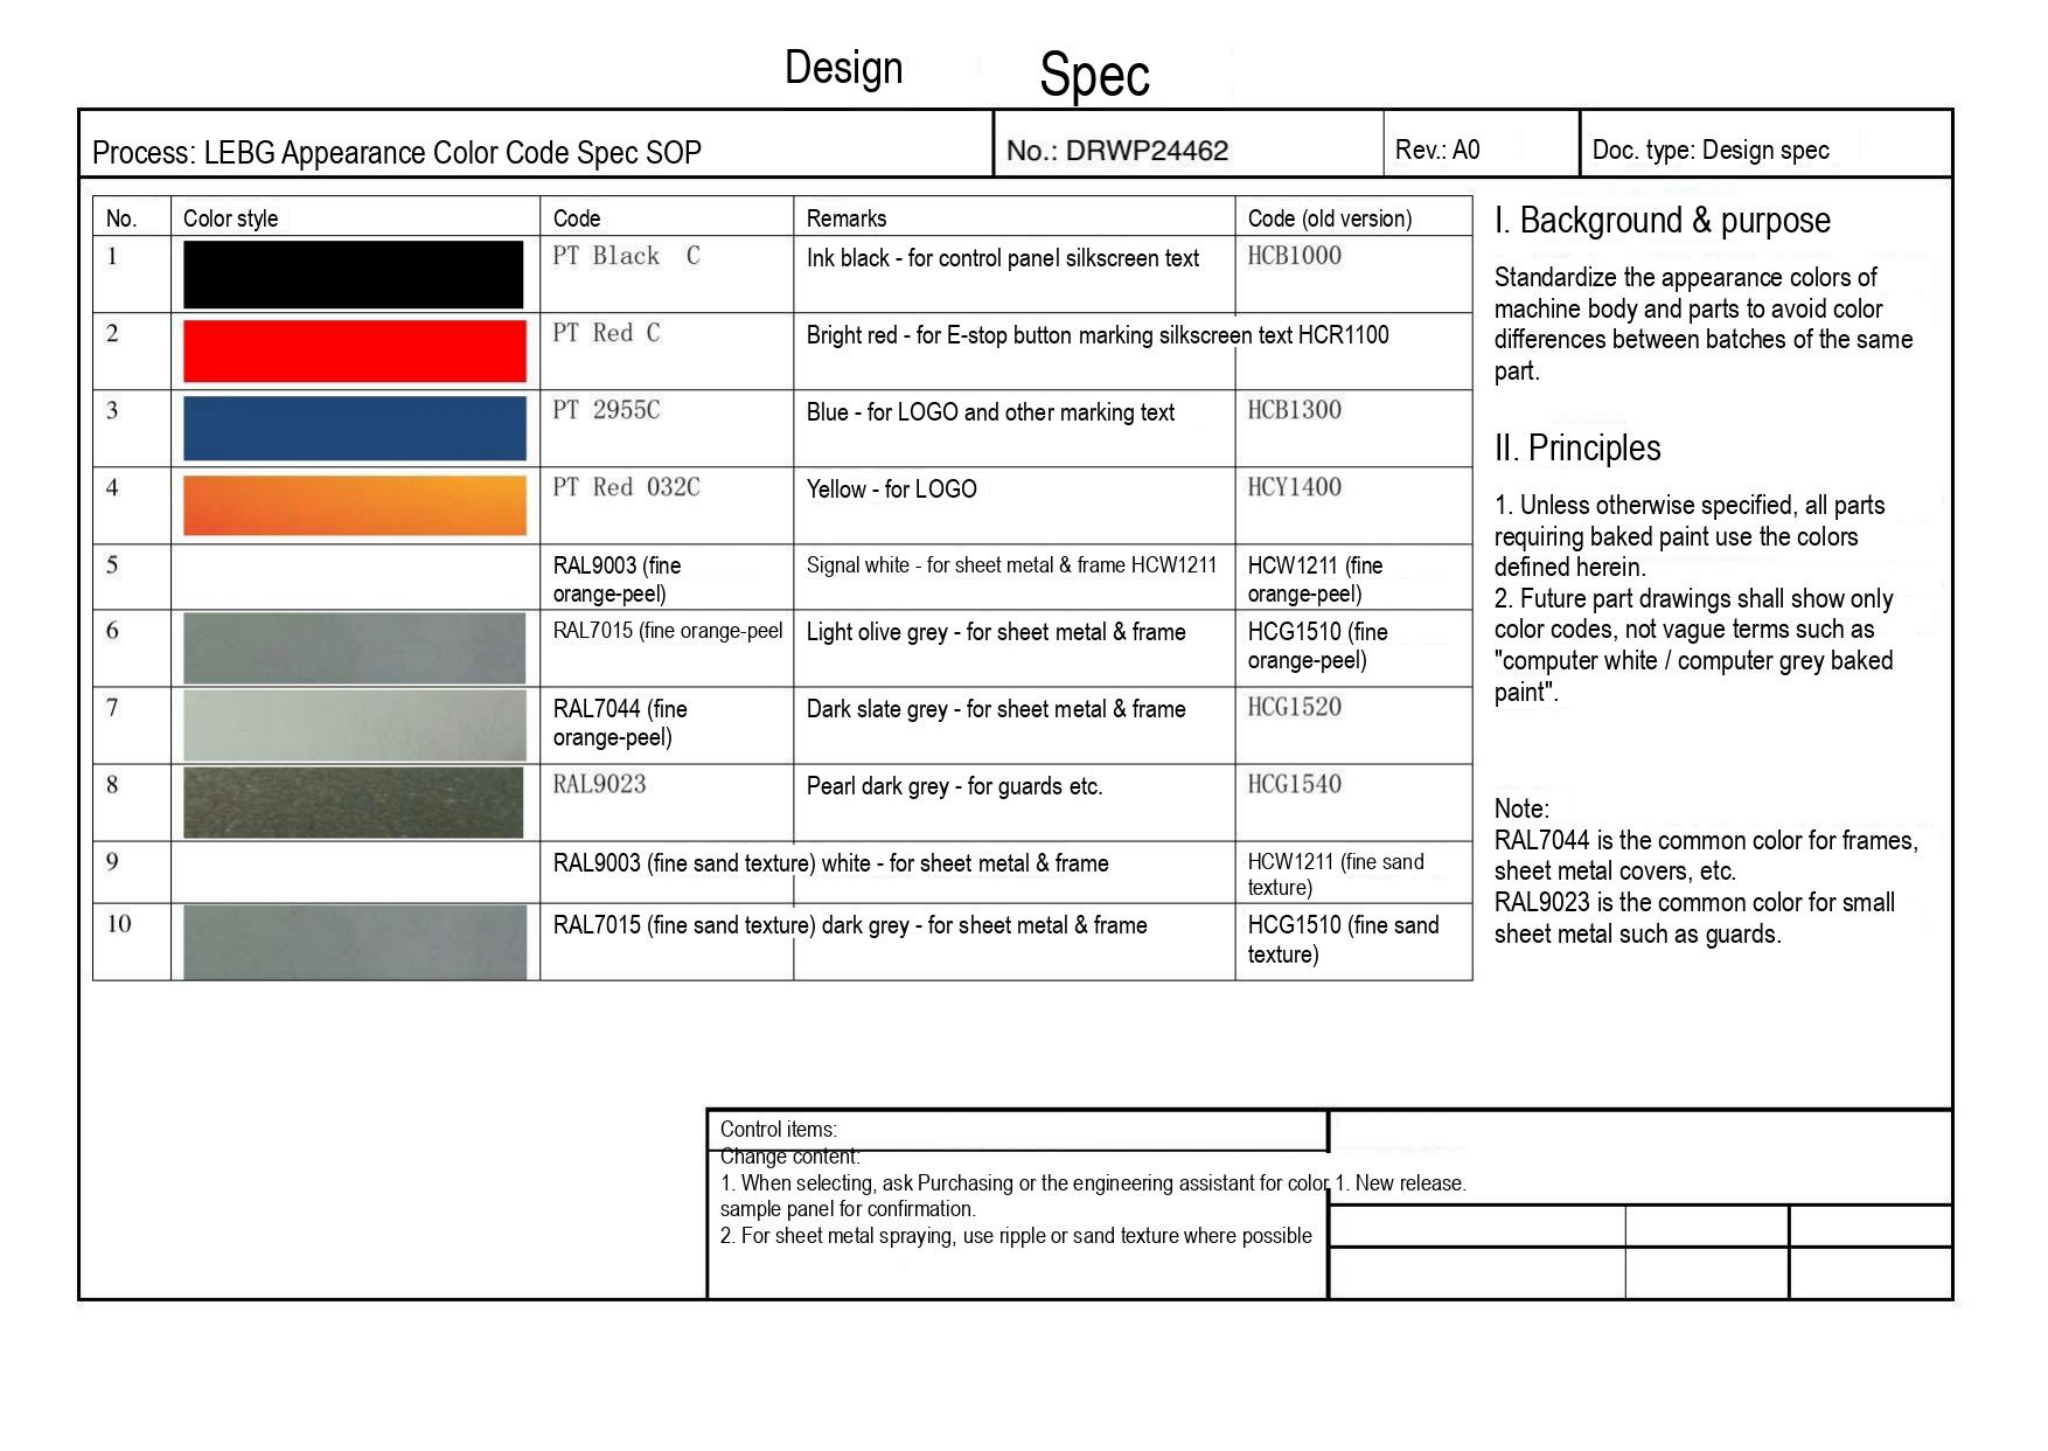Design Spec

| Process: LEBG Appearance Color Code Spec SOP | No.: DRWP24462 | Rev.: A0 | Doc. type: Design spec |
|---|---|---|---|

| No. | Color style | Code | Remarks | Code (old version) |
|---|---|---|---|---|
| 1 | | PT Black C | Ink black - for control panel silkscreen text | HCB1000 |
| 2 | | PT Red C | Bright red - for E-stop button marking silkscreen text HCR1100 | |
| 3 | | PT 2955C | Blue - for LOGO and other marking text | HCB1300 |
| 4 | | PT Red 032C | Yellow - for LOGO | HCY1400 |
| 5 | | RAL9003 (fine orange-peel) | Signal white - for sheet metal & frame HCW1211 | HCW1211 (fine orange-peel) |
| 6 | | RAL7015 (fine orange-peel | Light olive grey - for sheet metal & frame | HCG1510 (fine orange-peel) |
| 7 | | RAL7044 (fine orange-peel) | Dark slate grey - for sheet metal & frame | HCG1520 |
| 8 | | RAL9023 | Pearl dark grey - for guards etc. | HCG1540 |
| 9 | | RAL9003 (fine sand texture) white - for sheet metal & frame | | HCW1211 (fine sand texture) |
| 10 | | RAL7015 (fine sand texture) dark grey - for sheet metal & frame | | HCG1510 (fine sand texture) |

I. Background & purpose

Standardize the appearance colors of machine body and parts to avoid color differences between batches of the same part.

II. Principles

1. Unless otherwise specified, all parts requiring baked paint use the colors defined herein.
2. Future part drawings shall show only color codes, not vague terms such as "computer white / computer grey baked paint".

Note:
RAL7044 is the common color for frames, sheet metal covers, etc.
RAL9023 is the common color for small sheet metal such as guards.

Control items:
Change content:
1. When selecting, ask Purchasing or the engineering assistant for color sample panel for confirmation.
2. For sheet metal spraying, use ripple or sand texture where possible

1. New release.